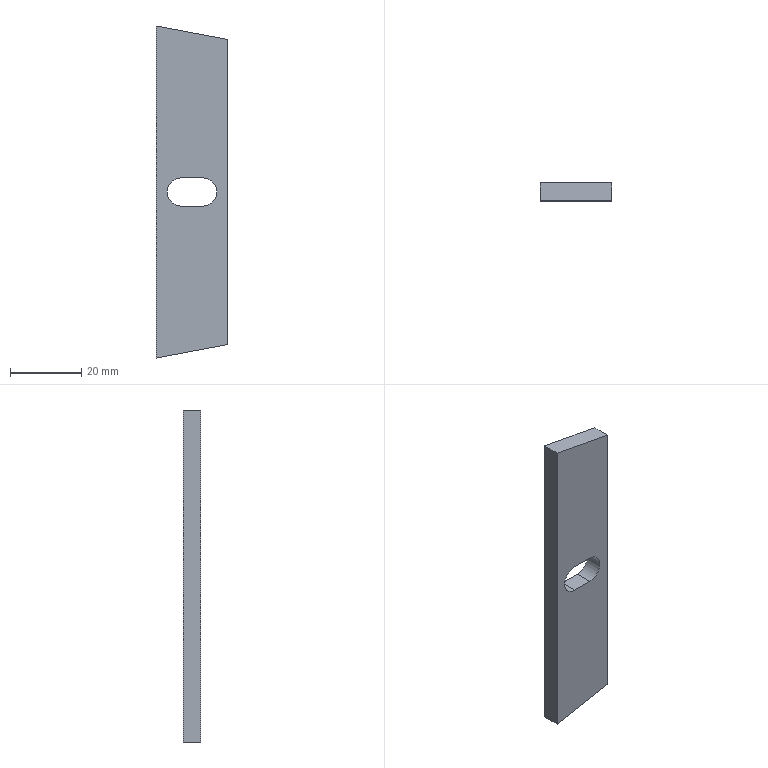Part | STEP file | PRT0001_68_19 | 1 solid | 10 faces | box 20 x 5 x 93.385 mm | volume 8469 mm3 | plane 8 | cylinder 2 | commonest cylinder face diameters 8 x2
STEP:
#1=CARTESIAN_POINT('',(0.,0.,0.));
#2=DIRECTION('',(0.,0.,1.));
#3=DIRECTION('',(1.,0.,0.));
#4=AXIS2_PLACEMENT_3D('',#1,#2,#3);
#5=CARTESIAN_POINT('',(1727.601,1237.457,-0.000000001));
#6=VERTEX_POINT('',#5);
#7=CARTESIAN_POINT('',(1731.601,1237.457,-4.));
#8=VERTEX_POINT('',#7);
#9=CARTESIAN_POINT('',(1731.601,1237.457,-0.000000001));
#10=DIRECTION('',(0.,-1.,0.));
#11=DIRECTION('',(-1.,0.,0.));
#12=AXIS2_PLACEMENT_3D('',#9,#10,#11);
#13=CIRCLE('',#12,4.);
#14=CARTESIAN_POINT('',(1731.601,1242.457,-0.000000001));
#15=DIRECTION('',(0.,1.,0.));
#16=DIRECTION('',(1.,0.,0.));
#17=AXIS2_PLACEMENT_3D('',#14,#15,#16);
#18=CYLINDRICAL_SURFACE('',#17,4.);
#19=CARTESIAN_POINT('',(3.142,-5.));
#20=DIRECTION('',(-1.,0.));
#21=VECTOR('',#20,1.);
#22=LINE('',#19,#21);
#23=(GEOMETRIC_REPRESENTATION_CONTEXT(2)PARAMETRIC_REPRESENTATION_CONTEXT()REPRESENTATION_CONTEXT('',''));
#24=DEFINITIONAL_REPRESENTATION('',(#22),#23);
#25=PCURVE('',#18,#24);
#26=CARTESIAN_POINT('',(1724.601,1237.457,72.014));
#27=DIRECTION('',(0.,-1.,0.));
#28=DIRECTION('',(1.,0.,0.));
#29=AXIS2_PLACEMENT_3D('',#26,#27,#28);
#30=PLANE('',#29);
#31=CARTESIAN_POINT('',(7.,-72.014));
#32=DIRECTION('',(-1.,0.));
#33=AXIS2_PLACEMENT_2D('',#31,#32);
#34=CIRCLE('',#33,4.);
#35=(GEOMETRIC_REPRESENTATION_CONTEXT(2)PARAMETRIC_REPRESENTATION_CONTEXT()REPRESENTATION_CONTEXT('',''));
#36=DEFINITIONAL_REPRESENTATION('',(#34),#35);
#37=PCURVE('',#30,#36);
#38=SURFACE_CURVE('',#13,(#25,#37),.PCURVE_S1.);
#39=EDGE_CURVE('',#6,#8,#38,.T.);
#40=ORIENTED_EDGE('',*,*,#39,.F.);
#41=CARTESIAN_POINT('',(1731.601,1237.457,4.));
#42=VERTEX_POINT('',#41);
#43=CARTESIAN_POINT('',(1731.601,1237.457,-0.000000001));
#44=DIRECTION('',(0.,-1.,0.));
#45=DIRECTION('',(0.,0.,1.));
#46=AXIS2_PLACEMENT_3D('',#43,#44,#45);
#47=CIRCLE('',#46,4.);
#48=CARTESIAN_POINT('',(4.712,-5.));
#49=DIRECTION('',(-1.,0.));
#50=VECTOR('',#49,1.);
#51=LINE('',#48,#50);
#52=(GEOMETRIC_REPRESENTATION_CONTEXT(2)PARAMETRIC_REPRESENTATION_CONTEXT()REPRESENTATION_CONTEXT('',''));
#53=DEFINITIONAL_REPRESENTATION('',(#51),#52);
#54=PCURVE('',#18,#53);
#55=CARTESIAN_POINT('',(7.,-72.014));
#56=DIRECTION('',(0.,1.));
#57=AXIS2_PLACEMENT_2D('',#55,#56);
#58=CIRCLE('',#57,4.);
#59=(GEOMETRIC_REPRESENTATION_CONTEXT(2)PARAMETRIC_REPRESENTATION_CONTEXT()REPRESENTATION_CONTEXT('',''));
#60=DEFINITIONAL_REPRESENTATION('',(#58),#59);
#61=PCURVE('',#30,#60);
#62=SURFACE_CURVE('',#47,(#54,#61),.PCURVE_S1.);
#63=EDGE_CURVE('',#42,#6,#62,.T.);
#64=ORIENTED_EDGE('',*,*,#63,.F.);
#65=CARTESIAN_POINT('',(1731.601,1242.457,4.));
#66=VERTEX_POINT('',#65);
#67=CARTESIAN_POINT('',(1731.601,1237.457,4.));
#68=DIRECTION('',(0.,1.,0.));
#69=VECTOR('',#68,1.);
#70=LINE('',#67,#69);
#71=CARTESIAN_POINT('',(4.712,-5.));
#72=DIRECTION('',(0.,1.));
#73=VECTOR('',#72,1.);
#74=LINE('',#71,#73);
#75=(GEOMETRIC_REPRESENTATION_CONTEXT(2)PARAMETRIC_REPRESENTATION_CONTEXT()REPRESENTATION_CONTEXT('',''));
#76=DEFINITIONAL_REPRESENTATION('',(#74),#75);
#77=PCURVE('',#18,#76);
#78=CARTESIAN_POINT('',(1731.601,1242.457,4.));
#79=DIRECTION('',(0.,0.,1.));
#80=DIRECTION('',(1.,0.,0.));
#81=AXIS2_PLACEMENT_3D('',#78,#79,#80);
#82=PLANE('',#81);
#83=CARTESIAN_POINT('',(0.,-5.));
#84=DIRECTION('',(0.,1.));
#85=VECTOR('',#84,1.);
#86=LINE('',#83,#85);
#87=(GEOMETRIC_REPRESENTATION_CONTEXT(2)PARAMETRIC_REPRESENTATION_CONTEXT()REPRESENTATION_CONTEXT('',''));
#88=DEFINITIONAL_REPRESENTATION('',(#86),#87);
#89=PCURVE('',#82,#88);
#90=SURFACE_CURVE('',#70,(#77,#89),.PCURVE_S1.);
#91=EDGE_CURVE('',#42,#66,#90,.T.);
#92=ORIENTED_EDGE('',*,*,#91,.T.);
#93=CARTESIAN_POINT('',(1727.601,1242.457,-0.000000001));
#94=VERTEX_POINT('',#93);
#95=CARTESIAN_POINT('',(1731.601,1242.457,-0.000000001));
#96=DIRECTION('',(0.,1.,0.));
#97=DIRECTION('',(-1.,0.,0.));
#98=AXIS2_PLACEMENT_3D('',#95,#96,#97);
#99=CIRCLE('',#98,4.);
#100=CARTESIAN_POINT('',(3.142,0.));
#101=DIRECTION('',(1.,0.));
#102=VECTOR('',#101,1.);
#103=LINE('',#100,#102);
#104=(GEOMETRIC_REPRESENTATION_CONTEXT(2)PARAMETRIC_REPRESENTATION_CONTEXT()REPRESENTATION_CONTEXT('',''));
#105=DEFINITIONAL_REPRESENTATION('',(#103),#104);
#106=PCURVE('',#18,#105);
#107=CARTESIAN_POINT('',(1744.601,1242.457,72.014));
#108=DIRECTION('',(0.,1.,0.));
#109=DIRECTION('',(-1.,0.,0.));
#110=AXIS2_PLACEMENT_3D('',#107,#108,#109);
#111=PLANE('',#110);
#112=CARTESIAN_POINT('',(13.,-72.014));
#113=DIRECTION('',(1.,0.));
#114=AXIS2_PLACEMENT_2D('',#112,#113);
#115=CIRCLE('',#114,4.);
#116=(GEOMETRIC_REPRESENTATION_CONTEXT(2)PARAMETRIC_REPRESENTATION_CONTEXT()REPRESENTATION_CONTEXT('',''));
#117=DEFINITIONAL_REPRESENTATION('',(#115),#116);
#118=PCURVE('',#111,#117);
#119=SURFACE_CURVE('',#99,(#106,#118),.PCURVE_S1.);
#120=EDGE_CURVE('',#94,#66,#119,.T.);
#121=ORIENTED_EDGE('',*,*,#120,.F.);
#122=CARTESIAN_POINT('',(1731.601,1242.457,-4.));
#123=VERTEX_POINT('',#122);
#124=CARTESIAN_POINT('',(1731.601,1242.457,-0.000000001));
#125=DIRECTION('',(0.,1.,0.));
#126=DIRECTION('',(0.,0.,-1.));
#127=AXIS2_PLACEMENT_3D('',#124,#125,#126);
#128=CIRCLE('',#127,4.);
#129=CARTESIAN_POINT('',(1.571,0.));
#130=DIRECTION('',(1.,0.));
#131=VECTOR('',#130,1.);
#132=LINE('',#129,#131);
#133=(GEOMETRIC_REPRESENTATION_CONTEXT(2)PARAMETRIC_REPRESENTATION_CONTEXT()REPRESENTATION_CONTEXT('',''));
#134=DEFINITIONAL_REPRESENTATION('',(#132),#133);
#135=PCURVE('',#18,#134);
#136=CARTESIAN_POINT('',(13.,-72.014));
#137=DIRECTION('',(0.,-1.));
#138=AXIS2_PLACEMENT_2D('',#136,#137);
#139=CIRCLE('',#138,4.);
#140=(GEOMETRIC_REPRESENTATION_CONTEXT(2)PARAMETRIC_REPRESENTATION_CONTEXT()REPRESENTATION_CONTEXT('',''));
#141=DEFINITIONAL_REPRESENTATION('',(#139),#140);
#142=PCURVE('',#111,#141);
#143=SURFACE_CURVE('',#128,(#135,#142),.PCURVE_S1.);
#144=EDGE_CURVE('',#123,#94,#143,.T.);
#145=ORIENTED_EDGE('',*,*,#144,.F.);
#146=CARTESIAN_POINT('',(1731.601,1242.457,-4.));
#147=DIRECTION('',(0.,-1.,0.));
#148=VECTOR('',#147,1.);
#149=LINE('',#146,#148);
#150=CARTESIAN_POINT('',(1.571,0.));
#151=DIRECTION('',(0.,-1.));
#152=VECTOR('',#151,1.);
#153=LINE('',#150,#152);
#154=(GEOMETRIC_REPRESENTATION_CONTEXT(2)PARAMETRIC_REPRESENTATION_CONTEXT()REPRESENTATION_CONTEXT('',''));
#155=DEFINITIONAL_REPRESENTATION('',(#153),#154);
#156=PCURVE('',#18,#155);
#157=CARTESIAN_POINT('',(1737.601,1242.457,-4.));
#158=DIRECTION('',(0.,0.,-1.));
#159=DIRECTION('',(-1.,0.,0.));
#160=AXIS2_PLACEMENT_3D('',#157,#158,#159);
#161=PLANE('',#160);
#162=CARTESIAN_POINT('',(6.,0.));
#163=DIRECTION('',(0.,-1.));
#164=VECTOR('',#163,1.);
#165=LINE('',#162,#164);
#166=(GEOMETRIC_REPRESENTATION_CONTEXT(2)PARAMETRIC_REPRESENTATION_CONTEXT()REPRESENTATION_CONTEXT('',''));
#167=DEFINITIONAL_REPRESENTATION('',(#165),#166);
#168=PCURVE('',#161,#167);
#169=SURFACE_CURVE('',#149,(#156,#168),.PCURVE_S1.);
#170=EDGE_CURVE('',#123,#8,#169,.T.);
#171=ORIENTED_EDGE('',*,*,#170,.T.);
#172=EDGE_LOOP('',(#40,#64,#92,#121,#145,#171));
#173=FACE_BOUND('',#172,.F.);
#174=ADVANCED_FACE('',(#173),#18,.F.);
#175=CARTESIAN_POINT('',(1744.601,1237.457,-42.913));
#176=VERTEX_POINT('',#175);
#177=CARTESIAN_POINT('',(1724.601,1237.457,-46.692));
#178=VERTEX_POINT('',#177);
#179=CARTESIAN_POINT('',(1744.601,1237.457,-42.913));
#180=DIRECTION('',(-0.9826,0.,-0.1857));
#181=VECTOR('',#180,1.);
#182=LINE('',#179,#181);
#183=CARTESIAN_POINT('',(20.,-114.927));
#184=DIRECTION('',(-0.9826,-0.1857));
#185=VECTOR('',#184,1.);
#186=LINE('',#183,#185);
#187=(GEOMETRIC_REPRESENTATION_CONTEXT(2)PARAMETRIC_REPRESENTATION_CONTEXT()REPRESENTATION_CONTEXT('',''));
#188=DEFINITIONAL_REPRESENTATION('',(#186),#187);
#189=PCURVE('',#30,#188);
#190=CARTESIAN_POINT('',(1750.605,1107.827,-41.778));
#191=DIRECTION('',(0.1857,0.,-0.9826));
#192=DIRECTION('',(-0.9826,0.,-0.1857));
#193=AXIS2_PLACEMENT_3D('',#190,#191,#192);
#194=PLANE('',#193);
#195=CARTESIAN_POINT('',(6.109,129.63));
#196=DIRECTION('',(1.,0.));
#197=VECTOR('',#196,1.);
#198=LINE('',#195,#197);
#199=(GEOMETRIC_REPRESENTATION_CONTEXT(2)PARAMETRIC_REPRESENTATION_CONTEXT()REPRESENTATION_CONTEXT('',''));
#200=DEFINITIONAL_REPRESENTATION('',(#198),#199);
#201=PCURVE('',#194,#200);
#202=SURFACE_CURVE('',#182,(#189,#201),.PCURVE_S1.);
#203=EDGE_CURVE('',#176,#178,#202,.T.);
#204=ORIENTED_EDGE('',*,*,#203,.T.);
#205=CARTESIAN_POINT('',(1724.601,1237.457,46.692));
#206=VERTEX_POINT('',#205);
#207=CARTESIAN_POINT('',(1724.601,1237.457,46.692));
#208=DIRECTION('',(0.,0.,-1.));
#209=VECTOR('',#208,1.);
#210=LINE('',#207,#209);
#211=CARTESIAN_POINT('',(0.,-25.322));
#212=DIRECTION('',(0.,-1.));
#213=VECTOR('',#212,1.);
#214=LINE('',#211,#213);
#215=(GEOMETRIC_REPRESENTATION_CONTEXT(2)PARAMETRIC_REPRESENTATION_CONTEXT()REPRESENTATION_CONTEXT('',''));
#216=DEFINITIONAL_REPRESENTATION('',(#214),#215);
#217=PCURVE('',#30,#216);
#218=CARTESIAN_POINT('',(1724.601,1242.457,72.014));
#219=DIRECTION('',(-1.,0.,0.));
#220=DIRECTION('',(0.,-1.,0.));
#221=AXIS2_PLACEMENT_3D('',#218,#219,#220);
#222=PLANE('',#221);
#223=CARTESIAN_POINT('',(5.,-25.322));
#224=DIRECTION('',(0.,-1.));
#225=VECTOR('',#224,1.);
#226=LINE('',#223,#225);
#227=(GEOMETRIC_REPRESENTATION_CONTEXT(2)PARAMETRIC_REPRESENTATION_CONTEXT()REPRESENTATION_CONTEXT('',''));
#228=DEFINITIONAL_REPRESENTATION('',(#226),#227);
#229=PCURVE('',#222,#228);
#230=SURFACE_CURVE('',#210,(#217,#229),.PCURVE_S1.);
#231=EDGE_CURVE('',#206,#178,#230,.T.);
#232=ORIENTED_EDGE('',*,*,#231,.F.);
#233=CARTESIAN_POINT('',(1744.601,1237.457,42.913));
#234=VERTEX_POINT('',#233);
#235=CARTESIAN_POINT('',(1724.601,1237.457,46.692));
#236=DIRECTION('',(0.9826,0.,-0.1857));
#237=VECTOR('',#236,1.);
#238=LINE('',#235,#237);
#239=CARTESIAN_POINT('',(0.,-25.322));
#240=DIRECTION('',(0.9826,-0.1857));
#241=VECTOR('',#240,1.);
#242=LINE('',#239,#241);
#243=(GEOMETRIC_REPRESENTATION_CONTEXT(2)PARAMETRIC_REPRESENTATION_CONTEXT()REPRESENTATION_CONTEXT('',''));
#244=DEFINITIONAL_REPRESENTATION('',(#242),#243);
#245=PCURVE('',#30,#244);
#246=CARTESIAN_POINT('',(1605.102,1107.827,69.276));
#247=DIRECTION('',(0.1857,0.,0.9826));
#248=DIRECTION('',(0.9826,0.,-0.1857));
#249=AXIS2_PLACEMENT_3D('',#246,#247,#248);
#250=PLANE('',#249);
#251=CARTESIAN_POINT('',(121.615,129.63));
#252=DIRECTION('',(1.,0.));
#253=VECTOR('',#252,1.);
#254=LINE('',#251,#253);
#255=(GEOMETRIC_REPRESENTATION_CONTEXT(2)PARAMETRIC_REPRESENTATION_CONTEXT()REPRESENTATION_CONTEXT('',''));
#256=DEFINITIONAL_REPRESENTATION('',(#254),#255);
#257=PCURVE('',#250,#256);
#258=SURFACE_CURVE('',#238,(#245,#257),.PCURVE_S1.);
#259=EDGE_CURVE('',#206,#234,#258,.T.);
#260=ORIENTED_EDGE('',*,*,#259,.T.);
#261=CARTESIAN_POINT('',(1744.601,1237.457,42.913));
#262=DIRECTION('',(0.,0.,-1.));
#263=VECTOR('',#262,1.);
#264=LINE('',#261,#263);
#265=CARTESIAN_POINT('',(20.,-29.102));
#266=DIRECTION('',(0.,-1.));
#267=VECTOR('',#266,1.);
#268=LINE('',#265,#267);
#269=(GEOMETRIC_REPRESENTATION_CONTEXT(2)PARAMETRIC_REPRESENTATION_CONTEXT()REPRESENTATION_CONTEXT('',''));
#270=DEFINITIONAL_REPRESENTATION('',(#268),#269);
#271=PCURVE('',#30,#270);
#272=CARTESIAN_POINT('',(1744.601,1237.457,72.014));
#273=DIRECTION('',(1.,0.,0.));
#274=DIRECTION('',(0.,1.,0.));
#275=AXIS2_PLACEMENT_3D('',#272,#273,#274);
#276=PLANE('',#275);
#277=CARTESIAN_POINT('',(0.,-29.102));
#278=DIRECTION('',(0.,-1.));
#279=VECTOR('',#278,1.);
#280=LINE('',#277,#279);
#281=(GEOMETRIC_REPRESENTATION_CONTEXT(2)PARAMETRIC_REPRESENTATION_CONTEXT()REPRESENTATION_CONTEXT('',''));
#282=DEFINITIONAL_REPRESENTATION('',(#280),#281);
#283=PCURVE('',#276,#282);
#284=SURFACE_CURVE('',#264,(#271,#283),.PCURVE_S1.);
#285=EDGE_CURVE('',#234,#176,#284,.T.);
#286=ORIENTED_EDGE('',*,*,#285,.T.);
#287=EDGE_LOOP('',(#204,#232,#260,#286));
#288=FACE_BOUND('',#287,.F.);
#289=CARTESIAN_POINT('',(1737.601,1237.457,4.));
#290=VERTEX_POINT('',#289);
#291=CARTESIAN_POINT('',(1737.601,1237.457,4.));
#292=DIRECTION('',(-1.,0.,0.));
#293=VECTOR('',#292,1.);
#294=LINE('',#291,#293);
#295=CARTESIAN_POINT('',(13.,-68.014));
#296=DIRECTION('',(-1.,0.));
#297=VECTOR('',#296,1.);
#298=LINE('',#295,#297);
#299=(GEOMETRIC_REPRESENTATION_CONTEXT(2)PARAMETRIC_REPRESENTATION_CONTEXT()REPRESENTATION_CONTEXT('',''));
#300=DEFINITIONAL_REPRESENTATION('',(#298),#299);
#301=PCURVE('',#30,#300);
#302=CARTESIAN_POINT('',(6.,-5.));
#303=DIRECTION('',(-1.,0.));
#304=VECTOR('',#303,1.);
#305=LINE('',#302,#304);
#306=(GEOMETRIC_REPRESENTATION_CONTEXT(2)PARAMETRIC_REPRESENTATION_CONTEXT()REPRESENTATION_CONTEXT('',''));
#307=DEFINITIONAL_REPRESENTATION('',(#305),#306);
#308=PCURVE('',#82,#307);
#309=SURFACE_CURVE('',#294,(#301,#308),.PCURVE_S1.);
#310=EDGE_CURVE('',#290,#42,#309,.T.);
#311=ORIENTED_EDGE('',*,*,#310,.T.);
#312=ORIENTED_EDGE('',*,*,#63,.T.);
#313=ORIENTED_EDGE('',*,*,#39,.T.);
#314=CARTESIAN_POINT('',(1737.601,1237.457,-4.));
#315=VERTEX_POINT('',#314);
#316=CARTESIAN_POINT('',(1731.601,1237.457,-4.));
#317=DIRECTION('',(1.,0.,0.));
#318=VECTOR('',#317,1.);
#319=LINE('',#316,#318);
#320=CARTESIAN_POINT('',(7.,-76.014));
#321=DIRECTION('',(1.,0.));
#322=VECTOR('',#321,1.);
#323=LINE('',#320,#322);
#324=(GEOMETRIC_REPRESENTATION_CONTEXT(2)PARAMETRIC_REPRESENTATION_CONTEXT()REPRESENTATION_CONTEXT('',''));
#325=DEFINITIONAL_REPRESENTATION('',(#323),#324);
#326=PCURVE('',#30,#325);
#327=CARTESIAN_POINT('',(6.,-5.));
#328=DIRECTION('',(-1.,0.));
#329=VECTOR('',#328,1.);
#330=LINE('',#327,#329);
#331=(GEOMETRIC_REPRESENTATION_CONTEXT(2)PARAMETRIC_REPRESENTATION_CONTEXT()REPRESENTATION_CONTEXT('',''));
#332=DEFINITIONAL_REPRESENTATION('',(#330),#331);
#333=PCURVE('',#161,#332);
#334=SURFACE_CURVE('',#319,(#326,#333),.PCURVE_S1.);
#335=EDGE_CURVE('',#8,#315,#334,.T.);
#336=ORIENTED_EDGE('',*,*,#335,.T.);
#337=CARTESIAN_POINT('',(1741.601,1237.457,-0.000000001));
#338=VERTEX_POINT('',#337);
#339=CARTESIAN_POINT('',(1737.601,1237.457,-0.000000001));
#340=DIRECTION('',(0.,-1.,0.));
#341=DIRECTION('',(0.,0.,-1.));
#342=AXIS2_PLACEMENT_3D('',#339,#340,#341);
#343=CIRCLE('',#342,4.);
#344=CARTESIAN_POINT('',(13.,-72.014));
#345=DIRECTION('',(0.,-1.));
#346=AXIS2_PLACEMENT_2D('',#344,#345);
#347=CIRCLE('',#346,4.);
#348=(GEOMETRIC_REPRESENTATION_CONTEXT(2)PARAMETRIC_REPRESENTATION_CONTEXT()REPRESENTATION_CONTEXT('',''));
#349=DEFINITIONAL_REPRESENTATION('',(#347),#348);
#350=PCURVE('',#30,#349);
#351=CARTESIAN_POINT('',(1737.601,1242.457,-0.000000001));
#352=DIRECTION('',(0.,1.,0.));
#353=DIRECTION('',(1.,0.,0.));
#354=AXIS2_PLACEMENT_3D('',#351,#352,#353);
#355=CYLINDRICAL_SURFACE('',#354,4.);
#356=CARTESIAN_POINT('',(1.571,-5.));
#357=DIRECTION('',(-1.,0.));
#358=VECTOR('',#357,1.);
#359=LINE('',#356,#358);
#360=(GEOMETRIC_REPRESENTATION_CONTEXT(2)PARAMETRIC_REPRESENTATION_CONTEXT()REPRESENTATION_CONTEXT('',''));
#361=DEFINITIONAL_REPRESENTATION('',(#359),#360);
#362=PCURVE('',#355,#361);
#363=SURFACE_CURVE('',#343,(#350,#362),.PCURVE_S1.);
#364=EDGE_CURVE('',#315,#338,#363,.T.);
#365=ORIENTED_EDGE('',*,*,#364,.T.);
#366=CARTESIAN_POINT('',(1737.601,1237.457,-0.000000001));
#367=DIRECTION('',(0.,-1.,0.));
#368=DIRECTION('',(1.,0.,0.));
#369=AXIS2_PLACEMENT_3D('',#366,#367,#368);
#370=CIRCLE('',#369,4.);
#371=CARTESIAN_POINT('',(13.,-72.014));
#372=DIRECTION('',(1.,0.));
#373=AXIS2_PLACEMENT_2D('',#371,#372);
#374=CIRCLE('',#373,4.);
#375=(GEOMETRIC_REPRESENTATION_CONTEXT(2)PARAMETRIC_REPRESENTATION_CONTEXT()REPRESENTATION_CONTEXT('',''));
#376=DEFINITIONAL_REPRESENTATION('',(#374),#375);
#377=PCURVE('',#30,#376);
#378=CARTESIAN_POINT('',(0.,-5.));
#379=DIRECTION('',(-1.,0.));
#380=VECTOR('',#379,1.);
#381=LINE('',#378,#380);
#382=(GEOMETRIC_REPRESENTATION_CONTEXT(2)PARAMETRIC_REPRESENTATION_CONTEXT()REPRESENTATION_CONTEXT('',''));
#383=DEFINITIONAL_REPRESENTATION('',(#381),#382);
#384=PCURVE('',#355,#383);
#385=SURFACE_CURVE('',#370,(#377,#384),.PCURVE_S1.);
#386=EDGE_CURVE('',#338,#290,#385,.T.);
#387=ORIENTED_EDGE('',*,*,#386,.T.);
#388=EDGE_LOOP('',(#311,#312,#313,#336,#365,#387));
#389=FACE_BOUND('',#388,.F.);
#390=ADVANCED_FACE('',(#288,#389),#30,.T.);
#391=CARTESIAN_POINT('',(1724.601,1242.457,-46.692));
#392=VERTEX_POINT('',#391);
#393=CARTESIAN_POINT('',(1724.601,1237.457,-46.692));
#394=DIRECTION('',(0.,1.,0.));
#395=VECTOR('',#394,1.);
#396=LINE('',#393,#395);
#397=CARTESIAN_POINT('',(26.463,129.63));
#398=DIRECTION('',(0.,1.));
#399=VECTOR('',#398,1.);
#400=LINE('',#397,#399);
#401=(GEOMETRIC_REPRESENTATION_CONTEXT(2)PARAMETRIC_REPRESENTATION_CONTEXT()REPRESENTATION_CONTEXT('',''));
#402=DEFINITIONAL_REPRESENTATION('',(#400),#401);
#403=PCURVE('',#194,#402);
#404=CARTESIAN_POINT('',(5.,-118.707));
#405=DIRECTION('',(-1.,0.));
#406=VECTOR('',#405,1.);
#407=LINE('',#404,#406);
#408=(GEOMETRIC_REPRESENTATION_CONTEXT(2)PARAMETRIC_REPRESENTATION_CONTEXT()REPRESENTATION_CONTEXT('',''));
#409=DEFINITIONAL_REPRESENTATION('',(#407),#408);
#410=PCURVE('',#222,#409);
#411=SURFACE_CURVE('',#396,(#403,#410),.PCURVE_S1.);
#412=EDGE_CURVE('',#178,#392,#411,.T.);
#413=ORIENTED_EDGE('',*,*,#412,.F.);
#414=ORIENTED_EDGE('',*,*,#203,.F.);
#415=CARTESIAN_POINT('',(1744.601,1242.457,-42.913));
#416=VERTEX_POINT('',#415);
#417=CARTESIAN_POINT('',(1744.601,1242.457,-42.913));
#418=DIRECTION('',(0.,-1.,0.));
#419=VECTOR('',#418,1.);
#420=LINE('',#417,#419);
#421=CARTESIAN_POINT('',(6.109,134.63));
#422=DIRECTION('',(0.,-1.));
#423=VECTOR('',#422,1.);
#424=LINE('',#421,#423);
#425=(GEOMETRIC_REPRESENTATION_CONTEXT(2)PARAMETRIC_REPRESENTATION_CONTEXT()REPRESENTATION_CONTEXT('',''));
#426=DEFINITIONAL_REPRESENTATION('',(#424),#425);
#427=PCURVE('',#194,#426);
#428=CARTESIAN_POINT('',(5.,-114.927));
#429=DIRECTION('',(-1.,0.));
#430=VECTOR('',#429,1.);
#431=LINE('',#428,#430);
#432=(GEOMETRIC_REPRESENTATION_CONTEXT(2)PARAMETRIC_REPRESENTATION_CONTEXT()REPRESENTATION_CONTEXT('',''));
#433=DEFINITIONAL_REPRESENTATION('',(#431),#432);
#434=PCURVE('',#276,#433);
#435=SURFACE_CURVE('',#420,(#427,#434),.PCURVE_S1.);
#436=EDGE_CURVE('',#416,#176,#435,.T.);
#437=ORIENTED_EDGE('',*,*,#436,.F.);
#438=CARTESIAN_POINT('',(1724.601,1242.457,-46.692));
#439=DIRECTION('',(0.9826,0.,0.1857));
#440=VECTOR('',#439,1.);
#441=LINE('',#438,#440);
#442=CARTESIAN_POINT('',(26.463,134.63));
#443=DIRECTION('',(-1.,0.));
#444=VECTOR('',#443,1.);
#445=LINE('',#442,#444);
#446=(GEOMETRIC_REPRESENTATION_CONTEXT(2)PARAMETRIC_REPRESENTATION_CONTEXT()REPRESENTATION_CONTEXT('',''));
#447=DEFINITIONAL_REPRESENTATION('',(#445),#446);
#448=PCURVE('',#194,#447);
#449=CARTESIAN_POINT('',(20.,-118.707));
#450=DIRECTION('',(-0.9826,0.1857));
#451=VECTOR('',#450,1.);
#452=LINE('',#449,#451);
#453=(GEOMETRIC_REPRESENTATION_CONTEXT(2)PARAMETRIC_REPRESENTATION_CONTEXT()REPRESENTATION_CONTEXT('',''));
#454=DEFINITIONAL_REPRESENTATION('',(#452),#453);
#455=PCURVE('',#111,#454);
#456=SURFACE_CURVE('',#441,(#448,#455),.PCURVE_S1.);
#457=EDGE_CURVE('',#392,#416,#456,.T.);
#458=ORIENTED_EDGE('',*,*,#457,.F.);
#459=EDGE_LOOP('',(#413,#414,#437,#458));
#460=FACE_BOUND('',#459,.F.);
#461=ADVANCED_FACE('',(#460),#194,.T.);
#462=ORIENTED_EDGE('',*,*,#412,.T.);
#463=CARTESIAN_POINT('',(1724.601,1242.457,46.692));
#464=VERTEX_POINT('',#463);
#465=CARTESIAN_POINT('',(1724.601,1242.457,46.692));
#466=DIRECTION('',(0.,0.,-1.));
#467=VECTOR('',#466,1.);
#468=LINE('',#465,#467);
#469=CARTESIAN_POINT('',(0.,-25.322));
#470=DIRECTION('',(0.,-1.));
#471=VECTOR('',#470,1.);
#472=LINE('',#469,#471);
#473=(GEOMETRIC_REPRESENTATION_CONTEXT(2)PARAMETRIC_REPRESENTATION_CONTEXT()REPRESENTATION_CONTEXT('',''));
#474=DEFINITIONAL_REPRESENTATION('',(#472),#473);
#475=PCURVE('',#222,#474);
#476=CARTESIAN_POINT('',(20.,-25.322));
#477=DIRECTION('',(0.,-1.));
#478=VECTOR('',#477,1.);
#479=LINE('',#476,#478);
#480=(GEOMETRIC_REPRESENTATION_CONTEXT(2)PARAMETRIC_REPRESENTATION_CONTEXT()REPRESENTATION_CONTEXT('',''));
#481=DEFINITIONAL_REPRESENTATION('',(#479),#480);
#482=PCURVE('',#111,#481);
#483=SURFACE_CURVE('',#468,(#475,#482),.PCURVE_S1.);
#484=EDGE_CURVE('',#464,#392,#483,.T.);
#485=ORIENTED_EDGE('',*,*,#484,.F.);
#486=CARTESIAN_POINT('',(1724.601,1237.457,46.692));
#487=DIRECTION('',(0.,1.,0.));
#488=VECTOR('',#487,1.);
#489=LINE('',#486,#488);
#490=CARTESIAN_POINT('',(5.,-25.322));
#491=DIRECTION('',(-1.,0.));
#492=VECTOR('',#491,1.);
#493=LINE('',#490,#492);
#494=(GEOMETRIC_REPRESENTATION_CONTEXT(2)PARAMETRIC_REPRESENTATION_CONTEXT()REPRESENTATION_CONTEXT('',''));
#495=DEFINITIONAL_REPRESENTATION('',(#493),#494);
#496=PCURVE('',#222,#495);
#497=CARTESIAN_POINT('',(121.615,129.63));
#498=DIRECTION('',(0.,1.));
#499=VECTOR('',#498,1.);
#500=LINE('',#497,#499);
#501=(GEOMETRIC_REPRESENTATION_CONTEXT(2)PARAMETRIC_REPRESENTATION_CONTEXT()REPRESENTATION_CONTEXT('',''));
#502=DEFINITIONAL_REPRESENTATION('',(#500),#501);
#503=PCURVE('',#250,#502);
#504=SURFACE_CURVE('',#489,(#496,#503),.PCURVE_S1.);
#505=EDGE_CURVE('',#206,#464,#504,.T.);
#506=ORIENTED_EDGE('',*,*,#505,.F.);
#507=ORIENTED_EDGE('',*,*,#231,.T.);
#508=EDGE_LOOP('',(#462,#485,#506,#507));
#509=FACE_BOUND('',#508,.F.);
#510=ADVANCED_FACE('',(#509),#222,.T.);
#511=ORIENTED_EDGE('',*,*,#457,.T.);
#512=CARTESIAN_POINT('',(1744.601,1242.457,42.913));
#513=VERTEX_POINT('',#512);
#514=CARTESIAN_POINT('',(1744.601,1242.457,42.913));
#515=DIRECTION('',(0.,0.,-1.));
#516=VECTOR('',#515,1.);
#517=LINE('',#514,#516);
#518=CARTESIAN_POINT('',(0.,-29.102));
#519=DIRECTION('',(0.,-1.));
#520=VECTOR('',#519,1.);
#521=LINE('',#518,#520);
#522=(GEOMETRIC_REPRESENTATION_CONTEXT(2)PARAMETRIC_REPRESENTATION_CONTEXT()REPRESENTATION_CONTEXT('',''));
#523=DEFINITIONAL_REPRESENTATION('',(#521),#522);
#524=PCURVE('',#111,#523);
#525=CARTESIAN_POINT('',(5.,-29.102));
#526=DIRECTION('',(0.,-1.));
#527=VECTOR('',#526,1.);
#528=LINE('',#525,#527);
#529=(GEOMETRIC_REPRESENTATION_CONTEXT(2)PARAMETRIC_REPRESENTATION_CONTEXT()REPRESENTATION_CONTEXT('',''));
#530=DEFINITIONAL_REPRESENTATION('',(#528),#529);
#531=PCURVE('',#276,#530);
#532=SURFACE_CURVE('',#517,(#524,#531),.PCURVE_S1.);
#533=EDGE_CURVE('',#513,#416,#532,.T.);
#534=ORIENTED_EDGE('',*,*,#533,.F.);
#535=CARTESIAN_POINT('',(1744.601,1242.457,42.913));
#536=DIRECTION('',(-0.9826,0.,0.1857));
#537=VECTOR('',#536,1.);
#538=LINE('',#535,#537);
#539=CARTESIAN_POINT('',(0.,-29.102));
#540=DIRECTION('',(0.9826,0.1857));
#541=VECTOR('',#540,1.);
#542=LINE('',#539,#541);
#543=(GEOMETRIC_REPRESENTATION_CONTEXT(2)PARAMETRIC_REPRESENTATION_CONTEXT()REPRESENTATION_CONTEXT('',''));
#544=DEFINITIONAL_REPRESENTATION('',(#542),#543);
#545=PCURVE('',#111,#544);
#546=CARTESIAN_POINT('',(141.969,134.63));
#547=DIRECTION('',(-1.,0.));
#548=VECTOR('',#547,1.);
#549=LINE('',#546,#548);
#550=(GEOMETRIC_REPRESENTATION_CONTEXT(2)PARAMETRIC_REPRESENTATION_CONTEXT()REPRESENTATION_CONTEXT('',''));
#551=DEFINITIONAL_REPRESENTATION('',(#549),#550);
#552=PCURVE('',#250,#551);
#553=SURFACE_CURVE('',#538,(#545,#552),.PCURVE_S1.);
#554=EDGE_CURVE('',#513,#464,#553,.T.);
#555=ORIENTED_EDGE('',*,*,#554,.T.);
#556=ORIENTED_EDGE('',*,*,#484,.T.);
#557=EDGE_LOOP('',(#511,#534,#555,#556));
#558=FACE_BOUND('',#557,.F.);
#559=CARTESIAN_POINT('',(1737.601,1242.457,4.));
#560=VERTEX_POINT('',#559);
#561=CARTESIAN_POINT('',(1737.601,1242.457,4.));
#562=DIRECTION('',(-1.,0.,0.));
#563=VECTOR('',#562,1.);
#564=LINE('',#561,#563);
#565=CARTESIAN_POINT('',(7.,-68.014));
#566=DIRECTION('',(1.,0.));
#567=VECTOR('',#566,1.);
#568=LINE('',#565,#567);
#569=(GEOMETRIC_REPRESENTATION_CONTEXT(2)PARAMETRIC_REPRESENTATION_CONTEXT()REPRESENTATION_CONTEXT('',''));
#570=DEFINITIONAL_REPRESENTATION('',(#568),#569);
#571=PCURVE('',#111,#570);
#572=CARTESIAN_POINT('',(6.,0.));
#573=DIRECTION('',(-1.,0.));
#574=VECTOR('',#573,1.);
#575=LINE('',#572,#574);
#576=(GEOMETRIC_REPRESENTATION_CONTEXT(2)PARAMETRIC_REPRESENTATION_CONTEXT()REPRESENTATION_CONTEXT('',''));
#577=DEFINITIONAL_REPRESENTATION('',(#575),#576);
#578=PCURVE('',#82,#577);
#579=SURFACE_CURVE('',#564,(#571,#578),.PCURVE_S1.);
#580=EDGE_CURVE('',#560,#66,#579,.T.);
#581=ORIENTED_EDGE('',*,*,#580,.F.);
#582=CARTESIAN_POINT('',(1741.601,1242.457,-0.000000001));
#583=VERTEX_POINT('',#582);
#584=CARTESIAN_POINT('',(1737.601,1242.457,-0.000000001));
#585=DIRECTION('',(0.,1.,0.));
#586=DIRECTION('',(0.,0.,1.));
#587=AXIS2_PLACEMENT_3D('',#584,#585,#586);
#588=CIRCLE('',#587,4.);
#589=CARTESIAN_POINT('',(7.,-72.014));
#590=DIRECTION('',(0.,1.));
#591=AXIS2_PLACEMENT_2D('',#589,#590);
#592=CIRCLE('',#591,4.);
#593=(GEOMETRIC_REPRESENTATION_CONTEXT(2)PARAMETRIC_REPRESENTATION_CONTEXT()REPRESENTATION_CONTEXT('',''));
#594=DEFINITIONAL_REPRESENTATION('',(#592),#593);
#595=PCURVE('',#111,#594);
#596=CARTESIAN_POINT('',(-1.571,0.));
#597=DIRECTION('',(1.,0.));
#598=VECTOR('',#597,1.);
#599=LINE('',#596,#598);
#600=(GEOMETRIC_REPRESENTATION_CONTEXT(2)PARAMETRIC_REPRESENTATION_CONTEXT()REPRESENTATION_CONTEXT('',''));
#601=DEFINITIONAL_REPRESENTATION('',(#599),#600);
#602=PCURVE('',#355,#601);
#603=SURFACE_CURVE('',#588,(#595,#602),.PCURVE_S1.);
#604=EDGE_CURVE('',#560,#583,#603,.T.);
#605=ORIENTED_EDGE('',*,*,#604,.T.);
#606=CARTESIAN_POINT('',(1737.601,1242.457,-4.));
#607=VERTEX_POINT('',#606);
#608=CARTESIAN_POINT('',(1737.601,1242.457,-0.000000001));
#609=DIRECTION('',(0.,1.,0.));
#610=DIRECTION('',(1.,0.,0.));
#611=AXIS2_PLACEMENT_3D('',#608,#609,#610);
#612=CIRCLE('',#611,4.);
#613=CARTESIAN_POINT('',(7.,-72.014));
#614=DIRECTION('',(-1.,0.));
#615=AXIS2_PLACEMENT_2D('',#613,#614);
#616=CIRCLE('',#615,4.);
#617=(GEOMETRIC_REPRESENTATION_CONTEXT(2)PARAMETRIC_REPRESENTATION_CONTEXT()REPRESENTATION_CONTEXT('',''));
#618=DEFINITIONAL_REPRESENTATION('',(#616),#617);
#619=PCURVE('',#111,#618);
#620=CARTESIAN_POINT('',(0.,0.));
#621=DIRECTION('',(1.,0.));
#622=VECTOR('',#621,1.);
#623=LINE('',#620,#622);
#624=(GEOMETRIC_REPRESENTATION_CONTEXT(2)PARAMETRIC_REPRESENTATION_CONTEXT()REPRESENTATION_CONTEXT('',''));
#625=DEFINITIONAL_REPRESENTATION('',(#623),#624);
#626=PCURVE('',#355,#625);
#627=SURFACE_CURVE('',#612,(#619,#626),.PCURVE_S1.);
#628=EDGE_CURVE('',#583,#607,#627,.T.);
#629=ORIENTED_EDGE('',*,*,#628,.T.);
#630=CARTESIAN_POINT('',(1731.601,1242.457,-4.));
#631=DIRECTION('',(1.,0.,0.));
#632=VECTOR('',#631,1.);
#633=LINE('',#630,#632);
#634=CARTESIAN_POINT('',(13.,-76.014));
#635=DIRECTION('',(-1.,0.));
#636=VECTOR('',#635,1.);
#637=LINE('',#634,#636);
#638=(GEOMETRIC_REPRESENTATION_CONTEXT(2)PARAMETRIC_REPRESENTATION_CONTEXT()REPRESENTATION_CONTEXT('',''));
#639=DEFINITIONAL_REPRESENTATION('',(#637),#638);
#640=PCURVE('',#111,#639);
#641=CARTESIAN_POINT('',(6.,0.));
#642=DIRECTION('',(-1.,0.));
#643=VECTOR('',#642,1.);
#644=LINE('',#641,#643);
#645=(GEOMETRIC_REPRESENTATION_CONTEXT(2)PARAMETRIC_REPRESENTATION_CONTEXT()REPRESENTATION_CONTEXT('',''));
#646=DEFINITIONAL_REPRESENTATION('',(#644),#645);
#647=PCURVE('',#161,#646);
#648=SURFACE_CURVE('',#633,(#640,#647),.PCURVE_S1.);
#649=EDGE_CURVE('',#123,#607,#648,.T.);
#650=ORIENTED_EDGE('',*,*,#649,.F.);
#651=ORIENTED_EDGE('',*,*,#144,.T.);
#652=ORIENTED_EDGE('',*,*,#120,.T.);
#653=EDGE_LOOP('',(#581,#605,#629,#650,#651,#652));
#654=FACE_BOUND('',#653,.F.);
#655=ADVANCED_FACE('',(#558,#654),#111,.T.);
#656=ORIENTED_EDGE('',*,*,#436,.T.);
#657=ORIENTED_EDGE('',*,*,#285,.F.);
#658=CARTESIAN_POINT('',(1744.601,1242.457,42.913));
#659=DIRECTION('',(0.,-1.,0.));
#660=VECTOR('',#659,1.);
#661=LINE('',#658,#660);
#662=CARTESIAN_POINT('',(5.,-29.102));
#663=DIRECTION('',(-1.,0.));
#664=VECTOR('',#663,1.);
#665=LINE('',#662,#664);
#666=(GEOMETRIC_REPRESENTATION_CONTEXT(2)PARAMETRIC_REPRESENTATION_CONTEXT()REPRESENTATION_CONTEXT('',''));
#667=DEFINITIONAL_REPRESENTATION('',(#665),#666);
#668=PCURVE('',#276,#667);
#669=CARTESIAN_POINT('',(141.969,134.63));
#670=DIRECTION('',(0.,-1.));
#671=VECTOR('',#670,1.);
#672=LINE('',#669,#671);
#673=(GEOMETRIC_REPRESENTATION_CONTEXT(2)PARAMETRIC_REPRESENTATION_CONTEXT()REPRESENTATION_CONTEXT('',''));
#674=DEFINITIONAL_REPRESENTATION('',(#672),#673);
#675=PCURVE('',#250,#674);
#676=SURFACE_CURVE('',#661,(#668,#675),.PCURVE_S1.);
#677=EDGE_CURVE('',#513,#234,#676,.T.);
#678=ORIENTED_EDGE('',*,*,#677,.F.);
#679=ORIENTED_EDGE('',*,*,#533,.T.);
#680=EDGE_LOOP('',(#656,#657,#678,#679));
#681=FACE_BOUND('',#680,.F.);
#682=ADVANCED_FACE('',(#681),#276,.T.);
#683=ORIENTED_EDGE('',*,*,#505,.T.);
#684=ORIENTED_EDGE('',*,*,#554,.F.);
#685=ORIENTED_EDGE('',*,*,#677,.T.);
#686=ORIENTED_EDGE('',*,*,#259,.F.);
#687=EDGE_LOOP('',(#683,#684,#685,#686));
#688=FACE_BOUND('',#687,.F.);
#689=ADVANCED_FACE('',(#688),#250,.T.);
#690=ORIENTED_EDGE('',*,*,#310,.F.);
#691=CARTESIAN_POINT('',(1737.601,1242.457,4.));
#692=DIRECTION('',(0.,-1.,0.));
#693=VECTOR('',#692,1.);
#694=LINE('',#691,#693);
#695=CARTESIAN_POINT('',(6.,0.));
#696=DIRECTION('',(0.,-1.));
#697=VECTOR('',#696,1.);
#698=LINE('',#695,#697);
#699=(GEOMETRIC_REPRESENTATION_CONTEXT(2)PARAMETRIC_REPRESENTATION_CONTEXT()REPRESENTATION_CONTEXT('',''));
#700=DEFINITIONAL_REPRESENTATION('',(#698),#699);
#701=PCURVE('',#82,#700);
#702=CARTESIAN_POINT('',(-1.571,0.));
#703=DIRECTION('',(0.,-1.));
#704=VECTOR('',#703,1.);
#705=LINE('',#702,#704);
#706=(GEOMETRIC_REPRESENTATION_CONTEXT(2)PARAMETRIC_REPRESENTATION_CONTEXT()REPRESENTATION_CONTEXT('',''));
#707=DEFINITIONAL_REPRESENTATION('',(#705),#706);
#708=PCURVE('',#355,#707);
#709=SURFACE_CURVE('',#694,(#701,#708),.PCURVE_S1.);
#710=EDGE_CURVE('',#560,#290,#709,.T.);
#711=ORIENTED_EDGE('',*,*,#710,.F.);
#712=ORIENTED_EDGE('',*,*,#580,.T.);
#713=ORIENTED_EDGE('',*,*,#91,.F.);
#714=EDGE_LOOP('',(#690,#711,#712,#713));
#715=FACE_BOUND('',#714,.F.);
#716=ADVANCED_FACE('',(#715),#82,.F.);
#717=ORIENTED_EDGE('',*,*,#386,.F.);
#718=ORIENTED_EDGE('',*,*,#364,.F.);
#719=CARTESIAN_POINT('',(1737.601,1237.457,-4.));
#720=DIRECTION('',(0.,1.,0.));
#721=VECTOR('',#720,1.);
#722=LINE('',#719,#721);
#723=CARTESIAN_POINT('',(1.571,-5.));
#724=DIRECTION('',(0.,1.));
#725=VECTOR('',#724,1.);
#726=LINE('',#723,#725);
#727=(GEOMETRIC_REPRESENTATION_CONTEXT(2)PARAMETRIC_REPRESENTATION_CONTEXT()REPRESENTATION_CONTEXT('',''));
#728=DEFINITIONAL_REPRESENTATION('',(#726),#727);
#729=PCURVE('',#355,#728);
#730=CARTESIAN_POINT('',(0.,-5.));
#731=DIRECTION('',(0.,1.));
#732=VECTOR('',#731,1.);
#733=LINE('',#730,#732);
#734=(GEOMETRIC_REPRESENTATION_CONTEXT(2)PARAMETRIC_REPRESENTATION_CONTEXT()REPRESENTATION_CONTEXT('',''));
#735=DEFINITIONAL_REPRESENTATION('',(#733),#734);
#736=PCURVE('',#161,#735);
#737=SURFACE_CURVE('',#722,(#729,#736),.PCURVE_S1.);
#738=EDGE_CURVE('',#315,#607,#737,.T.);
#739=ORIENTED_EDGE('',*,*,#738,.T.);
#740=ORIENTED_EDGE('',*,*,#628,.F.);
#741=ORIENTED_EDGE('',*,*,#604,.F.);
#742=ORIENTED_EDGE('',*,*,#710,.T.);
#743=EDGE_LOOP('',(#717,#718,#739,#740,#741,#742));
#744=FACE_BOUND('',#743,.F.);
#745=ADVANCED_FACE('',(#744),#355,.F.);
#746=ORIENTED_EDGE('',*,*,#335,.F.);
#747=ORIENTED_EDGE('',*,*,#170,.F.);
#748=ORIENTED_EDGE('',*,*,#649,.T.);
#749=ORIENTED_EDGE('',*,*,#738,.F.);
#750=EDGE_LOOP('',(#746,#747,#748,#749));
#751=FACE_BOUND('',#750,.F.);
#752=ADVANCED_FACE('',(#751),#161,.F.);
#753=CLOSED_SHELL('',(#174,#390,#461,#510,#655,#682,#689,#716,#745,#752));
#754=MANIFOLD_SOLID_BREP('',#753);
#755=(LENGTH_UNIT()NAMED_UNIT(*)SI_UNIT(.MILLI.,.METRE.));
#756=UNCERTAINTY_MEASURE_WITH_UNIT(LENGTH_MEASURE(0.0000001),#755,'','');
#757=(NAMED_UNIT(*)PLANE_ANGLE_UNIT()SI_UNIT($,.RADIAN.));
#758=(NAMED_UNIT(*)SI_UNIT($,.STERADIAN.)SOLID_ANGLE_UNIT());
#759=(GEOMETRIC_REPRESENTATION_CONTEXT(3)GLOBAL_UNCERTAINTY_ASSIGNED_CONTEXT((#756))GLOBAL_UNIT_ASSIGNED_CONTEXT((#755,#757,#758))REPRESENTATION_CONTEXT('',''));
#760=ADVANCED_BREP_SHAPE_REPRESENTATION('',(#4,#754),#759);